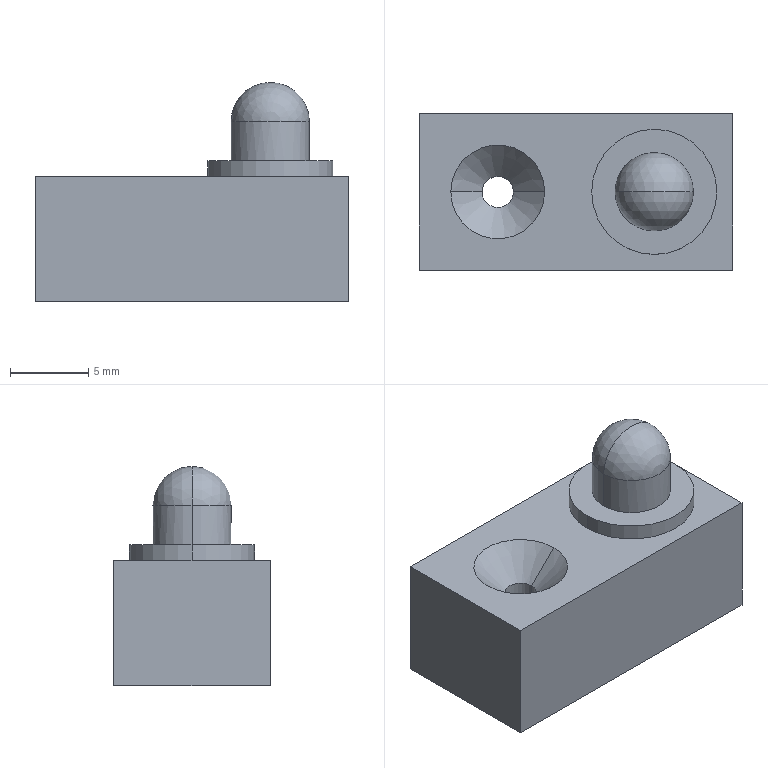Part | SolidWorks | features ICE 3, Chamfer 1, Extrusion 1, Fillet 1 | 1 solid | 17 faces | box 20 x 10 x 14 mm | volume 1686 mm3 | plane 7 | cylinder 6 | sphere 2 | cone 2 | commonest cylinder face diameters 2 x2 5 x2 8 x2
STEP:
#1=CARTESIAN_POINT('',(12.5,5.,11.5));
#2=VERTEX_POINT('',#1);
#3=CARTESIAN_POINT('',(17.5,5.,11.5));
#4=VERTEX_POINT('',#3);
#5=CARTESIAN_POINT('',(15.,5.,11.5));
#6=DIRECTION('',(0.,0.,-1.));
#7=DIRECTION('',(-1.,0.,0.));
#8=AXIS2_PLACEMENT_3D('',#5,#6,#7);
#9=CIRCLE('',#8,2.5);
#10=EDGE_CURVE('',#2,#4,#9,.T.);
#11=ORIENTED_EDGE('',*,*,#10,.F.);
#12=CARTESIAN_POINT('',(15.,5.,14.));
#13=VERTEX_POINT('',#12);
#14=CARTESIAN_POINT('',(15.,5.,11.5));
#15=DIRECTION('',(0.,1.,0.));
#16=DIRECTION('',(-1.,0.,0.));
#17=AXIS2_PLACEMENT_3D('',#14,#15,#16);
#18=CIRCLE('',#17,2.5);
#19=EDGE_CURVE('',#2,#13,#18,.T.);
#20=ORIENTED_EDGE('',*,*,#19,.T.);
#21=CARTESIAN_POINT('',(15.,5.,11.5));
#22=DIRECTION('',(0.,-1.,0.));
#23=DIRECTION('',(0.,0.,-1.));
#24=AXIS2_PLACEMENT_3D('',#21,#22,#23);
#25=CIRCLE('',#24,2.5);
#26=EDGE_CURVE('',#4,#13,#25,.T.);
#27=ORIENTED_EDGE('',*,*,#26,.F.);
#28=EDGE_LOOP('',(#11,#20,#27));
#29=FACE_OUTER_BOUND('',#28,.T.);
#30=CARTESIAN_POINT('',(15.,5.,11.5));
#31=DIRECTION('',(0.,1.,0.));
#32=DIRECTION('',(1.,0.,0.));
#33=AXIS2_PLACEMENT_3D('',#30,#31,#32);
#34=SPHERICAL_SURFACE('',#33,2.5);
#35=ADVANCED_FACE('',(#29),#34,.T.);
#36=ORIENTED_EDGE('',*,*,#10,.T.);
#37=CARTESIAN_POINT('',(17.5,5.,9.));
#38=VERTEX_POINT('',#37);
#39=CARTESIAN_POINT('',(17.5,5.,14.));
#40=DIRECTION('',(0.,0.,-1.));
#41=VECTOR('',#40,1000.);
#42=LINE('',#39,#41);
#43=EDGE_CURVE('',#4,#38,#42,.T.);
#44=ORIENTED_EDGE('',*,*,#43,.T.);
#45=CARTESIAN_POINT('',(12.5,5.,9.));
#46=VERTEX_POINT('',#45);
#47=CARTESIAN_POINT('',(15.,5.,9.));
#48=DIRECTION('',(0.,0.,1.));
#49=DIRECTION('',(1.,0.,0.));
#50=AXIS2_PLACEMENT_3D('',#47,#48,#49);
#51=CIRCLE('',#50,2.5);
#52=EDGE_CURVE('',#38,#46,#51,.T.);
#53=ORIENTED_EDGE('',*,*,#52,.T.);
#54=CARTESIAN_POINT('',(12.5,5.,14.));
#55=DIRECTION('',(0.,0.,-1.));
#56=VECTOR('',#55,1000.);
#57=LINE('',#54,#56);
#58=EDGE_CURVE('',#2,#46,#57,.T.);
#59=ORIENTED_EDGE('',*,*,#58,.F.);
#60=EDGE_LOOP('',(#36,#44,#53,#59));
#61=FACE_OUTER_BOUND('',#60,.T.);
#62=CARTESIAN_POINT('',(15.,5.,14.));
#63=DIRECTION('',(0.,0.,-1.));
#64=DIRECTION('',(-1.,0.,0.));
#65=AXIS2_PLACEMENT_3D('',#62,#63,#64);
#66=CYLINDRICAL_SURFACE('',#65,2.5);
#67=ADVANCED_FACE('',(#61),#66,.T.);
#68=CARTESIAN_POINT('',(19.,5.,9.));
#69=VERTEX_POINT('',#68);
#70=CARTESIAN_POINT('',(11.,5.,9.));
#71=VERTEX_POINT('',#70);
#72=CARTESIAN_POINT('',(15.,5.,9.));
#73=DIRECTION('',(0.,0.,1.));
#74=DIRECTION('',(1.,0.,0.));
#75=AXIS2_PLACEMENT_3D('',#72,#73,#74);
#76=CIRCLE('',#75,4.);
#77=EDGE_CURVE('',#69,#71,#76,.T.);
#78=ORIENTED_EDGE('',*,*,#77,.F.);
#79=CARTESIAN_POINT('',(19.,5.,8.));
#80=VERTEX_POINT('',#79);
#81=CARTESIAN_POINT('',(19.,5.,9.));
#82=DIRECTION('',(0.,0.,-1.));
#83=VECTOR('',#82,1000.);
#84=LINE('',#81,#83);
#85=EDGE_CURVE('',#69,#80,#84,.T.);
#86=ORIENTED_EDGE('',*,*,#85,.T.);
#87=CARTESIAN_POINT('',(11.,5.,8.));
#88=VERTEX_POINT('',#87);
#89=CARTESIAN_POINT('',(15.,5.,8.));
#90=DIRECTION('',(0.,0.,1.));
#91=DIRECTION('',(-1.,0.,0.));
#92=AXIS2_PLACEMENT_3D('',#89,#90,#91);
#93=CIRCLE('',#92,4.);
#94=EDGE_CURVE('',#80,#88,#93,.T.);
#95=ORIENTED_EDGE('',*,*,#94,.T.);
#96=CARTESIAN_POINT('',(11.,5.,9.));
#97=DIRECTION('',(0.,0.,-1.));
#98=VECTOR('',#97,1000.);
#99=LINE('',#96,#98);
#100=EDGE_CURVE('',#71,#88,#99,.T.);
#101=ORIENTED_EDGE('',*,*,#100,.F.);
#102=EDGE_LOOP('',(#78,#86,#95,#101));
#103=FACE_OUTER_BOUND('',#102,.T.);
#104=CARTESIAN_POINT('',(15.,5.,9.));
#105=DIRECTION('',(0.,0.,-1.));
#106=DIRECTION('',(-1.,0.,0.));
#107=AXIS2_PLACEMENT_3D('',#104,#105,#106);
#108=CYLINDRICAL_SURFACE('',#107,4.);
#109=ADVANCED_FACE('',(#103),#108,.T.);
#110=CARTESIAN_POINT('',(4.,5.,6.));
#111=VERTEX_POINT('',#110);
#112=CARTESIAN_POINT('',(6.,5.,6.));
#113=VERTEX_POINT('',#112);
#114=CARTESIAN_POINT('',(5.,5.,6.));
#115=DIRECTION('',(0.,0.,1.));
#116=DIRECTION('',(-1.,0.,0.));
#117=AXIS2_PLACEMENT_3D('',#114,#115,#116);
#118=CIRCLE('',#117,1.);
#119=EDGE_CURVE('',#111,#113,#118,.T.);
#120=ORIENTED_EDGE('',*,*,#119,.F.);
#121=CARTESIAN_POINT('',(2.,5.,8.));
#122=VERTEX_POINT('',#121);
#123=CARTESIAN_POINT('',(4.,5.,6.));
#124=DIRECTION('',(-0.7071,0.,0.7071));
#125=VECTOR('',#124,1000.);
#126=LINE('',#123,#125);
#127=EDGE_CURVE('',#111,#122,#126,.T.);
#128=ORIENTED_EDGE('',*,*,#127,.T.);
#129=CARTESIAN_POINT('',(8.,5.,8.));
#130=VERTEX_POINT('',#129);
#131=CARTESIAN_POINT('',(5.,5.,8.));
#132=DIRECTION('',(0.,0.,-1.));
#133=DIRECTION('',(-1.,0.,0.));
#134=AXIS2_PLACEMENT_3D('',#131,#132,#133);
#135=CIRCLE('',#134,3.);
#136=EDGE_CURVE('',#130,#122,#135,.T.);
#137=ORIENTED_EDGE('',*,*,#136,.F.);
#138=CARTESIAN_POINT('',(6.,5.,6.));
#139=DIRECTION('',(0.7071,0.,0.7071));
#140=VECTOR('',#139,1000.);
#141=LINE('',#138,#140);
#142=EDGE_CURVE('',#113,#130,#141,.T.);
#143=ORIENTED_EDGE('',*,*,#142,.F.);
#144=EDGE_LOOP('',(#120,#128,#137,#143));
#145=FACE_OUTER_BOUND('',#144,.T.);
#146=CARTESIAN_POINT('',(5.,5.,6.));
#147=DIRECTION('',(0.,0.,1.));
#148=DIRECTION('',(1.,0.,0.));
#149=AXIS2_PLACEMENT_3D('',#146,#147,#148);
#150=CONICAL_SURFACE('',#149,1.,0.7854);
#151=ADVANCED_FACE('',(#145),#150,.F.);
#152=CARTESIAN_POINT('',(4.,5.,0.));
#153=VERTEX_POINT('',#152);
#154=CARTESIAN_POINT('',(6.,5.,0.));
#155=VERTEX_POINT('',#154);
#156=CARTESIAN_POINT('',(5.,5.,0.));
#157=DIRECTION('',(0.,0.,1.));
#158=DIRECTION('',(1.,0.,0.));
#159=AXIS2_PLACEMENT_3D('',#156,#157,#158);
#160=CIRCLE('',#159,1.);
#161=EDGE_CURVE('',#153,#155,#160,.T.);
#162=ORIENTED_EDGE('',*,*,#161,.F.);
#163=CARTESIAN_POINT('',(4.,5.,0.));
#164=DIRECTION('',(0.,0.,1.));
#165=VECTOR('',#164,1000.);
#166=LINE('',#163,#165);
#167=EDGE_CURVE('',#153,#111,#166,.T.);
#168=ORIENTED_EDGE('',*,*,#167,.T.);
#169=ORIENTED_EDGE('',*,*,#119,.T.);
#170=CARTESIAN_POINT('',(6.,5.,0.));
#171=DIRECTION('',(0.,0.,1.));
#172=VECTOR('',#171,1000.);
#173=LINE('',#170,#172);
#174=EDGE_CURVE('',#155,#113,#173,.T.);
#175=ORIENTED_EDGE('',*,*,#174,.F.);
#176=EDGE_LOOP('',(#162,#168,#169,#175));
#177=FACE_OUTER_BOUND('',#176,.T.);
#178=CARTESIAN_POINT('',(5.,5.,0.));
#179=DIRECTION('',(0.,0.,1.));
#180=DIRECTION('',(1.,0.,0.));
#181=AXIS2_PLACEMENT_3D('',#178,#179,#180);
#182=CYLINDRICAL_SURFACE('',#181,1.);
#183=ADVANCED_FACE('',(#177),#182,.F.);
#184=CARTESIAN_POINT('',(0.,10.,0.));
#185=VERTEX_POINT('',#184);
#186=CARTESIAN_POINT('',(0.,0.,0.));
#187=VERTEX_POINT('',#186);
#188=CARTESIAN_POINT('',(0.,0.,0.));
#189=DIRECTION('',(0.,-1.,0.));
#190=VECTOR('',#189,1000.);
#191=LINE('',#188,#190);
#192=EDGE_CURVE('',#185,#187,#191,.T.);
#193=ORIENTED_EDGE('',*,*,#192,.T.);
#194=CARTESIAN_POINT('',(0.,0.,8.));
#195=VERTEX_POINT('',#194);
#196=CARTESIAN_POINT('',(0.,0.,8.));
#197=DIRECTION('',(0.,0.,-1.));
#198=VECTOR('',#197,1000.);
#199=LINE('',#196,#198);
#200=EDGE_CURVE('',#195,#187,#199,.T.);
#201=ORIENTED_EDGE('',*,*,#200,.F.);
#202=CARTESIAN_POINT('',(0.,10.,8.));
#203=VERTEX_POINT('',#202);
#204=CARTESIAN_POINT('',(0.,0.,8.));
#205=DIRECTION('',(0.,-1.,0.));
#206=VECTOR('',#205,1000.);
#207=LINE('',#204,#206);
#208=EDGE_CURVE('',#203,#195,#207,.T.);
#209=ORIENTED_EDGE('',*,*,#208,.F.);
#210=CARTESIAN_POINT('',(0.,10.,8.));
#211=DIRECTION('',(0.,0.,-1.));
#212=VECTOR('',#211,1000.);
#213=LINE('',#210,#212);
#214=EDGE_CURVE('',#203,#185,#213,.T.);
#215=ORIENTED_EDGE('',*,*,#214,.T.);
#216=EDGE_LOOP('',(#193,#201,#209,#215));
#217=FACE_OUTER_BOUND('',#216,.T.);
#218=CARTESIAN_POINT('',(0.,0.,8.));
#219=DIRECTION('',(1.,0.,0.));
#220=DIRECTION('',(0.,0.,-1.));
#221=AXIS2_PLACEMENT_3D('',#218,#219,#220);
#222=PLANE('',#221);
#223=ADVANCED_FACE('',(#217),#222,.F.);
#224=CARTESIAN_POINT('',(20.,0.,0.));
#225=VERTEX_POINT('',#224);
#226=CARTESIAN_POINT('',(0.,0.,0.));
#227=DIRECTION('',(1.,0.,0.));
#228=VECTOR('',#227,1000.);
#229=LINE('',#226,#228);
#230=EDGE_CURVE('',#187,#225,#229,.T.);
#231=ORIENTED_EDGE('',*,*,#230,.T.);
#232=CARTESIAN_POINT('',(20.,0.,8.));
#233=VERTEX_POINT('',#232);
#234=CARTESIAN_POINT('',(20.,0.,8.));
#235=DIRECTION('',(0.,0.,-1.));
#236=VECTOR('',#235,1000.);
#237=LINE('',#234,#236);
#238=EDGE_CURVE('',#233,#225,#237,.T.);
#239=ORIENTED_EDGE('',*,*,#238,.F.);
#240=CARTESIAN_POINT('',(0.,0.,8.));
#241=DIRECTION('',(1.,0.,0.));
#242=VECTOR('',#241,1000.);
#243=LINE('',#240,#242);
#244=EDGE_CURVE('',#195,#233,#243,.T.);
#245=ORIENTED_EDGE('',*,*,#244,.F.);
#246=ORIENTED_EDGE('',*,*,#200,.T.);
#247=EDGE_LOOP('',(#231,#239,#245,#246));
#248=FACE_OUTER_BOUND('',#247,.T.);
#249=CARTESIAN_POINT('',(0.,0.,8.));
#250=DIRECTION('',(0.,1.,0.));
#251=DIRECTION('',(0.,0.,1.));
#252=AXIS2_PLACEMENT_3D('',#249,#250,#251);
#253=PLANE('',#252);
#254=ADVANCED_FACE('',(#248),#253,.F.);
#255=CARTESIAN_POINT('',(20.,10.,0.));
#256=VERTEX_POINT('',#255);
#257=CARTESIAN_POINT('',(20.,0.,0.));
#258=DIRECTION('',(0.,1.,0.));
#259=VECTOR('',#258,1000.);
#260=LINE('',#257,#259);
#261=EDGE_CURVE('',#225,#256,#260,.T.);
#262=ORIENTED_EDGE('',*,*,#261,.T.);
#263=CARTESIAN_POINT('',(20.,10.,8.));
#264=VERTEX_POINT('',#263);
#265=CARTESIAN_POINT('',(20.,10.,8.));
#266=DIRECTION('',(0.,0.,-1.));
#267=VECTOR('',#266,1000.);
#268=LINE('',#265,#267);
#269=EDGE_CURVE('',#264,#256,#268,.T.);
#270=ORIENTED_EDGE('',*,*,#269,.F.);
#271=CARTESIAN_POINT('',(20.,0.,8.));
#272=DIRECTION('',(0.,1.,0.));
#273=VECTOR('',#272,1000.);
#274=LINE('',#271,#273);
#275=EDGE_CURVE('',#233,#264,#274,.T.);
#276=ORIENTED_EDGE('',*,*,#275,.F.);
#277=ORIENTED_EDGE('',*,*,#238,.T.);
#278=EDGE_LOOP('',(#262,#270,#276,#277));
#279=FACE_OUTER_BOUND('',#278,.T.);
#280=CARTESIAN_POINT('',(20.,0.,8.));
#281=DIRECTION('',(-1.,0.,0.));
#282=DIRECTION('',(0.,0.,1.));
#283=AXIS2_PLACEMENT_3D('',#280,#281,#282);
#284=PLANE('',#283);
#285=ADVANCED_FACE('',(#279),#284,.F.);
#286=CARTESIAN_POINT('',(0.,10.,0.));
#287=DIRECTION('',(-1.,0.,0.));
#288=VECTOR('',#287,1000.);
#289=LINE('',#286,#288);
#290=EDGE_CURVE('',#256,#185,#289,.T.);
#291=ORIENTED_EDGE('',*,*,#290,.T.);
#292=ORIENTED_EDGE('',*,*,#214,.F.);
#293=CARTESIAN_POINT('',(0.,10.,8.));
#294=DIRECTION('',(-1.,0.,0.));
#295=VECTOR('',#294,1000.);
#296=LINE('',#293,#295);
#297=EDGE_CURVE('',#264,#203,#296,.T.);
#298=ORIENTED_EDGE('',*,*,#297,.F.);
#299=ORIENTED_EDGE('',*,*,#269,.T.);
#300=EDGE_LOOP('',(#291,#292,#298,#299));
#301=FACE_OUTER_BOUND('',#300,.T.);
#302=CARTESIAN_POINT('',(0.,10.,8.));
#303=DIRECTION('',(0.,-1.,0.));
#304=DIRECTION('',(0.,0.,-1.));
#305=AXIS2_PLACEMENT_3D('',#302,#303,#304);
#306=PLANE('',#305);
#307=ADVANCED_FACE('',(#301),#306,.F.);
#308=CARTESIAN_POINT('',(15.,5.,8.));
#309=DIRECTION('',(0.,0.,1.));
#310=DIRECTION('',(-1.,0.,0.));
#311=AXIS2_PLACEMENT_3D('',#308,#309,#310);
#312=CIRCLE('',#311,4.);
#313=EDGE_CURVE('',#88,#80,#312,.T.);
#314=ORIENTED_EDGE('',*,*,#313,.F.);
#315=ORIENTED_EDGE('',*,*,#94,.F.);
#316=EDGE_LOOP('',(#314,#315));
#317=FACE_BOUND('',#316,.T.);
#318=ORIENTED_EDGE('',*,*,#136,.T.);
#319=CARTESIAN_POINT('',(5.,5.,8.));
#320=DIRECTION('',(0.,0.,-1.));
#321=DIRECTION('',(-1.,0.,0.));
#322=AXIS2_PLACEMENT_3D('',#319,#320,#321);
#323=CIRCLE('',#322,3.);
#324=EDGE_CURVE('',#122,#130,#323,.T.);
#325=ORIENTED_EDGE('',*,*,#324,.T.);
#326=EDGE_LOOP('',(#318,#325));
#327=FACE_BOUND('',#326,.T.);
#328=ORIENTED_EDGE('',*,*,#208,.T.);
#329=ORIENTED_EDGE('',*,*,#244,.T.);
#330=ORIENTED_EDGE('',*,*,#275,.T.);
#331=ORIENTED_EDGE('',*,*,#297,.T.);
#332=EDGE_LOOP('',(#328,#329,#330,#331));
#333=FACE_OUTER_BOUND('',#332,.T.);
#334=CARTESIAN_POINT('',(0.,0.,8.));
#335=DIRECTION('',(0.,0.,-1.));
#336=DIRECTION('',(-1.,0.,0.));
#337=AXIS2_PLACEMENT_3D('',#334,#335,#336);
#338=PLANE('',#337);
#339=ADVANCED_FACE('',(#317,#327,#333),#338,.F.);
#340=CARTESIAN_POINT('',(5.,5.,0.));
#341=DIRECTION('',(0.,0.,1.));
#342=DIRECTION('',(1.,0.,0.));
#343=AXIS2_PLACEMENT_3D('',#340,#341,#342);
#344=CIRCLE('',#343,1.);
#345=EDGE_CURVE('',#155,#153,#344,.T.);
#346=ORIENTED_EDGE('',*,*,#345,.T.);
#347=ORIENTED_EDGE('',*,*,#161,.T.);
#348=EDGE_LOOP('',(#346,#347));
#349=FACE_BOUND('',#348,.T.);
#350=ORIENTED_EDGE('',*,*,#192,.F.);
#351=ORIENTED_EDGE('',*,*,#290,.F.);
#352=ORIENTED_EDGE('',*,*,#261,.F.);
#353=ORIENTED_EDGE('',*,*,#230,.F.);
#354=EDGE_LOOP('',(#350,#351,#352,#353));
#355=FACE_OUTER_BOUND('',#354,.T.);
#356=CARTESIAN_POINT('',(0.,0.,0.));
#357=DIRECTION('',(0.,0.,-1.));
#358=DIRECTION('',(-1.,0.,0.));
#359=AXIS2_PLACEMENT_3D('',#356,#357,#358);
#360=PLANE('',#359);
#361=ADVANCED_FACE('',(#349,#355),#360,.T.);
#362=ORIENTED_EDGE('',*,*,#167,.F.);
#363=ORIENTED_EDGE('',*,*,#345,.F.);
#364=ORIENTED_EDGE('',*,*,#174,.T.);
#365=CARTESIAN_POINT('',(5.,5.,6.));
#366=DIRECTION('',(0.,0.,1.));
#367=DIRECTION('',(-1.,0.,0.));
#368=AXIS2_PLACEMENT_3D('',#365,#366,#367);
#369=CIRCLE('',#368,1.);
#370=EDGE_CURVE('',#113,#111,#369,.T.);
#371=ORIENTED_EDGE('',*,*,#370,.T.);
#372=EDGE_LOOP('',(#362,#363,#364,#371));
#373=FACE_OUTER_BOUND('',#372,.T.);
#374=CARTESIAN_POINT('',(5.,5.,0.));
#375=DIRECTION('',(0.,0.,1.));
#376=DIRECTION('',(1.,0.,0.));
#377=AXIS2_PLACEMENT_3D('',#374,#375,#376);
#378=CYLINDRICAL_SURFACE('',#377,1.);
#379=ADVANCED_FACE('',(#373),#378,.F.);
#380=ORIENTED_EDGE('',*,*,#127,.F.);
#381=ORIENTED_EDGE('',*,*,#370,.F.);
#382=ORIENTED_EDGE('',*,*,#142,.T.);
#383=ORIENTED_EDGE('',*,*,#324,.F.);
#384=EDGE_LOOP('',(#380,#381,#382,#383));
#385=FACE_OUTER_BOUND('',#384,.T.);
#386=CARTESIAN_POINT('',(5.,5.,6.));
#387=DIRECTION('',(0.,0.,1.));
#388=DIRECTION('',(1.,0.,0.));
#389=AXIS2_PLACEMENT_3D('',#386,#387,#388);
#390=CONICAL_SURFACE('',#389,1.,0.7854);
#391=ADVANCED_FACE('',(#385),#390,.F.);
#392=ORIENTED_EDGE('',*,*,#85,.F.);
#393=CARTESIAN_POINT('',(15.,5.,9.));
#394=DIRECTION('',(0.,0.,1.));
#395=DIRECTION('',(1.,0.,0.));
#396=AXIS2_PLACEMENT_3D('',#393,#394,#395);
#397=CIRCLE('',#396,4.);
#398=EDGE_CURVE('',#71,#69,#397,.T.);
#399=ORIENTED_EDGE('',*,*,#398,.F.);
#400=ORIENTED_EDGE('',*,*,#100,.T.);
#401=ORIENTED_EDGE('',*,*,#313,.T.);
#402=EDGE_LOOP('',(#392,#399,#400,#401));
#403=FACE_OUTER_BOUND('',#402,.T.);
#404=CARTESIAN_POINT('',(15.,5.,9.));
#405=DIRECTION('',(0.,0.,-1.));
#406=DIRECTION('',(-1.,0.,0.));
#407=AXIS2_PLACEMENT_3D('',#404,#405,#406);
#408=CYLINDRICAL_SURFACE('',#407,4.);
#409=ADVANCED_FACE('',(#403),#408,.T.);
#410=CARTESIAN_POINT('',(15.,5.,9.));
#411=DIRECTION('',(0.,0.,1.));
#412=DIRECTION('',(1.,0.,0.));
#413=AXIS2_PLACEMENT_3D('',#410,#411,#412);
#414=CIRCLE('',#413,2.5);
#415=EDGE_CURVE('',#46,#38,#414,.T.);
#416=ORIENTED_EDGE('',*,*,#415,.F.);
#417=ORIENTED_EDGE('',*,*,#52,.F.);
#418=EDGE_LOOP('',(#416,#417));
#419=FACE_BOUND('',#418,.T.);
#420=ORIENTED_EDGE('',*,*,#398,.T.);
#421=ORIENTED_EDGE('',*,*,#77,.T.);
#422=EDGE_LOOP('',(#420,#421));
#423=FACE_OUTER_BOUND('',#422,.T.);
#424=CARTESIAN_POINT('',(15.,5.,9.));
#425=DIRECTION('',(0.,0.,1.));
#426=DIRECTION('',(1.,0.,0.));
#427=AXIS2_PLACEMENT_3D('',#424,#425,#426);
#428=PLANE('',#427);
#429=ADVANCED_FACE('',(#419,#423),#428,.T.);
#430=ORIENTED_EDGE('',*,*,#43,.F.);
#431=CARTESIAN_POINT('',(15.,5.,11.5));
#432=DIRECTION('',(0.,0.,-1.));
#433=DIRECTION('',(-1.,0.,0.));
#434=AXIS2_PLACEMENT_3D('',#431,#432,#433);
#435=CIRCLE('',#434,2.5);
#436=EDGE_CURVE('',#4,#2,#435,.T.);
#437=ORIENTED_EDGE('',*,*,#436,.T.);
#438=ORIENTED_EDGE('',*,*,#58,.T.);
#439=ORIENTED_EDGE('',*,*,#415,.T.);
#440=EDGE_LOOP('',(#430,#437,#438,#439));
#441=FACE_OUTER_BOUND('',#440,.T.);
#442=CARTESIAN_POINT('',(15.,5.,14.));
#443=DIRECTION('',(0.,0.,-1.));
#444=DIRECTION('',(-1.,0.,0.));
#445=AXIS2_PLACEMENT_3D('',#442,#443,#444);
#446=CYLINDRICAL_SURFACE('',#445,2.5);
#447=ADVANCED_FACE('',(#441),#446,.T.);
#448=ORIENTED_EDGE('',*,*,#19,.F.);
#449=ORIENTED_EDGE('',*,*,#436,.F.);
#450=ORIENTED_EDGE('',*,*,#26,.T.);
#451=EDGE_LOOP('',(#448,#449,#450));
#452=FACE_OUTER_BOUND('',#451,.T.);
#453=CARTESIAN_POINT('',(15.,5.,11.5));
#454=DIRECTION('',(0.,1.,0.));
#455=DIRECTION('',(1.,0.,0.));
#456=AXIS2_PLACEMENT_3D('',#453,#454,#455);
#457=SPHERICAL_SURFACE('',#456,2.5);
#458=ADVANCED_FACE('',(#452),#457,.T.);
#459=CLOSED_SHELL('',(#35,#67,#109,#151,#183,#223,#254,#285,#307,#339,#361,#379,#391,#409,#429,#447,#458));
#460=MANIFOLD_SOLID_BREP('',#459);
#461=CARTESIAN_POINT('',(0.,0.,0.));
#462=DIRECTION('',(0.,0.,1.));
#463=DIRECTION('',(1.,0.,0.));
#464=AXIS2_PLACEMENT_3D('',#461,#462,#463);
#465=(LENGTH_UNIT()NAMED_UNIT(*)SI_UNIT(.MILLI.,.METRE.));
#466=UNCERTAINTY_MEASURE_WITH_UNIT(LENGTH_MEASURE(0.00001),#465,'','');
#467=(NAMED_UNIT(*)PLANE_ANGLE_UNIT()SI_UNIT($,.RADIAN.));
#468=(NAMED_UNIT(*)SI_UNIT($,.STERADIAN.)SOLID_ANGLE_UNIT());
#469=(GEOMETRIC_REPRESENTATION_CONTEXT(3)GLOBAL_UNCERTAINTY_ASSIGNED_CONTEXT((#466))GLOBAL_UNIT_ASSIGNED_CONTEXT((#465,#467,#468))REPRESENTATION_CONTEXT('',''));
#470=ADVANCED_BREP_SHAPE_REPRESENTATION('',(#460,#464),#469);